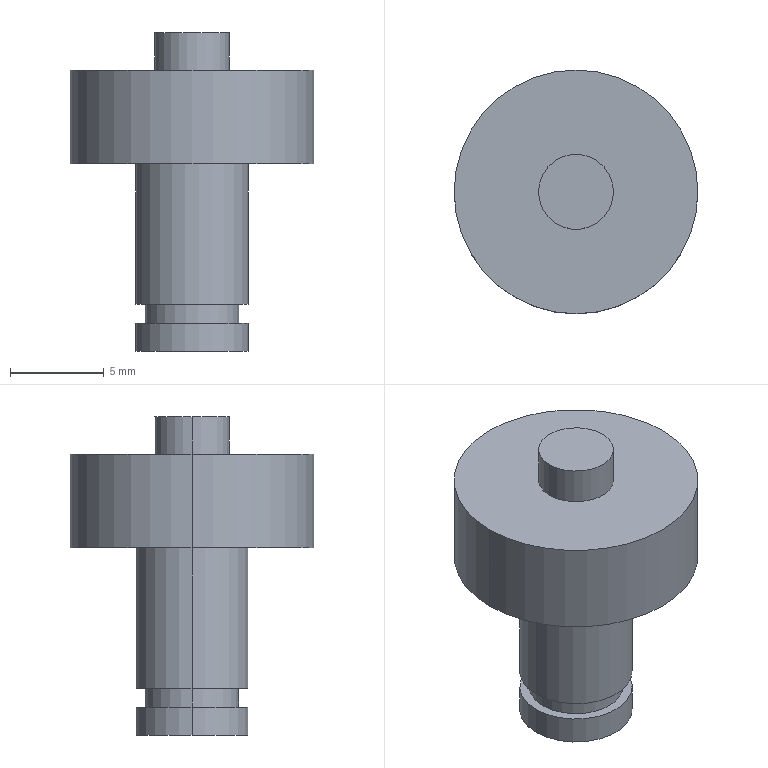Part | SolidWorks | features Boss 4, Extrusion 1 | 1 solid | 16 faces | box 13 x 13 x 17 mm | volume 962.898 mm3 | cylinder 10 | plane 6 | commonest cylinder face diameters 6 x4 4 x2 5 x2 13 x2
STEP:
#1=CARTESIAN_POINT('',(-3.,0.,-10.));
#2=VERTEX_POINT('',#1);
#3=CARTESIAN_POINT('',(3.,0.,-10.));
#4=VERTEX_POINT('',#3);
#5=CARTESIAN_POINT('',(0.,0.,-10.));
#6=DIRECTION('',(0.,0.,-1.));
#7=DIRECTION('',(-1.,0.,0.));
#8=AXIS2_PLACEMENT_3D('',#5,#6,#7);
#9=CIRCLE('',#8,3.);
#10=EDGE_CURVE('',#2,#4,#9,.T.);
#11=ORIENTED_EDGE('',*,*,#10,.F.);
#12=CARTESIAN_POINT('',(-3.,0.,-8.5));
#13=VERTEX_POINT('',#12);
#14=CARTESIAN_POINT('',(-3.,0.,-10.));
#15=DIRECTION('',(0.,0.,1.));
#16=VECTOR('',#15,1000.);
#17=LINE('',#14,#16);
#18=EDGE_CURVE('',#2,#13,#17,.T.);
#19=ORIENTED_EDGE('',*,*,#18,.T.);
#20=CARTESIAN_POINT('',(3.,0.,-8.5));
#21=VERTEX_POINT('',#20);
#22=CARTESIAN_POINT('',(0.,0.,-8.5));
#23=DIRECTION('',(0.,0.,-1.));
#24=DIRECTION('',(-1.,0.,0.));
#25=AXIS2_PLACEMENT_3D('',#22,#23,#24);
#26=CIRCLE('',#25,3.);
#27=EDGE_CURVE('',#13,#21,#26,.T.);
#28=ORIENTED_EDGE('',*,*,#27,.T.);
#29=CARTESIAN_POINT('',(3.,0.,-10.));
#30=DIRECTION('',(0.,0.,1.));
#31=VECTOR('',#30,1000.);
#32=LINE('',#29,#31);
#33=EDGE_CURVE('',#4,#21,#32,.T.);
#34=ORIENTED_EDGE('',*,*,#33,.F.);
#35=EDGE_LOOP('',(#11,#19,#28,#34));
#36=FACE_OUTER_BOUND('',#35,.T.);
#37=CARTESIAN_POINT('',(0.,0.,-10.));
#38=DIRECTION('',(0.,0.,1.));
#39=DIRECTION('',(1.,0.,0.));
#40=AXIS2_PLACEMENT_3D('',#37,#38,#39);
#41=CYLINDRICAL_SURFACE('',#40,3.);
#42=ADVANCED_FACE('',(#36),#41,.T.);
#43=CARTESIAN_POINT('',(-2.5,0.,-8.5));
#44=VERTEX_POINT('',#43);
#45=CARTESIAN_POINT('',(2.5,0.,-8.5));
#46=VERTEX_POINT('',#45);
#47=CARTESIAN_POINT('',(0.,0.,-8.5));
#48=DIRECTION('',(0.,0.,-1.));
#49=DIRECTION('',(-1.,0.,0.));
#50=AXIS2_PLACEMENT_3D('',#47,#48,#49);
#51=CIRCLE('',#50,2.5);
#52=EDGE_CURVE('',#44,#46,#51,.T.);
#53=ORIENTED_EDGE('',*,*,#52,.F.);
#54=CARTESIAN_POINT('',(-2.5,0.,-7.5));
#55=VERTEX_POINT('',#54);
#56=CARTESIAN_POINT('',(-2.5,0.,-8.5));
#57=DIRECTION('',(0.,0.,1.));
#58=VECTOR('',#57,1000.);
#59=LINE('',#56,#58);
#60=EDGE_CURVE('',#44,#55,#59,.T.);
#61=ORIENTED_EDGE('',*,*,#60,.T.);
#62=CARTESIAN_POINT('',(2.5,0.,-7.5));
#63=VERTEX_POINT('',#62);
#64=CARTESIAN_POINT('',(0.,0.,-7.5));
#65=DIRECTION('',(0.,0.,-1.));
#66=DIRECTION('',(-1.,0.,0.));
#67=AXIS2_PLACEMENT_3D('',#64,#65,#66);
#68=CIRCLE('',#67,2.5);
#69=EDGE_CURVE('',#55,#63,#68,.T.);
#70=ORIENTED_EDGE('',*,*,#69,.T.);
#71=CARTESIAN_POINT('',(2.5,0.,-8.5));
#72=DIRECTION('',(0.,0.,1.));
#73=VECTOR('',#72,1000.);
#74=LINE('',#71,#73);
#75=EDGE_CURVE('',#46,#63,#74,.T.);
#76=ORIENTED_EDGE('',*,*,#75,.F.);
#77=EDGE_LOOP('',(#53,#61,#70,#76));
#78=FACE_OUTER_BOUND('',#77,.T.);
#79=CARTESIAN_POINT('',(0.,0.,-8.5));
#80=DIRECTION('',(0.,0.,1.));
#81=DIRECTION('',(1.,0.,0.));
#82=AXIS2_PLACEMENT_3D('',#79,#80,#81);
#83=CYLINDRICAL_SURFACE('',#82,2.5);
#84=ADVANCED_FACE('',(#78),#83,.T.);
#85=CARTESIAN_POINT('',(-3.,0.,-7.5));
#86=VERTEX_POINT('',#85);
#87=CARTESIAN_POINT('',(3.,0.,-7.5));
#88=VERTEX_POINT('',#87);
#89=CARTESIAN_POINT('',(0.,0.,-7.5));
#90=DIRECTION('',(0.,0.,-1.));
#91=DIRECTION('',(-1.,0.,0.));
#92=AXIS2_PLACEMENT_3D('',#89,#90,#91);
#93=CIRCLE('',#92,3.);
#94=EDGE_CURVE('',#86,#88,#93,.T.);
#95=ORIENTED_EDGE('',*,*,#94,.F.);
#96=CARTESIAN_POINT('',(-3.,0.,0.));
#97=VERTEX_POINT('',#96);
#98=CARTESIAN_POINT('',(-3.,0.,-7.5));
#99=DIRECTION('',(0.,0.,1.));
#100=VECTOR('',#99,1000.);
#101=LINE('',#98,#100);
#102=EDGE_CURVE('',#86,#97,#101,.T.);
#103=ORIENTED_EDGE('',*,*,#102,.T.);
#104=CARTESIAN_POINT('',(3.,0.,0.));
#105=VERTEX_POINT('',#104);
#106=CARTESIAN_POINT('',(0.,0.,0.));
#107=DIRECTION('',(0.,0.,-1.));
#108=DIRECTION('',(1.,0.,0.));
#109=AXIS2_PLACEMENT_3D('',#106,#107,#108);
#110=CIRCLE('',#109,3.);
#111=EDGE_CURVE('',#97,#105,#110,.T.);
#112=ORIENTED_EDGE('',*,*,#111,.T.);
#113=CARTESIAN_POINT('',(3.,0.,-7.5));
#114=DIRECTION('',(0.,0.,1.));
#115=VECTOR('',#114,1000.);
#116=LINE('',#113,#115);
#117=EDGE_CURVE('',#88,#105,#116,.T.);
#118=ORIENTED_EDGE('',*,*,#117,.F.);
#119=EDGE_LOOP('',(#95,#103,#112,#118));
#120=FACE_OUTER_BOUND('',#119,.T.);
#121=CARTESIAN_POINT('',(0.,0.,-7.5));
#122=DIRECTION('',(0.,0.,1.));
#123=DIRECTION('',(1.,0.,0.));
#124=AXIS2_PLACEMENT_3D('',#121,#122,#123);
#125=CYLINDRICAL_SURFACE('',#124,3.);
#126=ADVANCED_FACE('',(#120),#125,.T.);
#127=CARTESIAN_POINT('',(2.,0.,7.));
#128=VERTEX_POINT('',#127);
#129=CARTESIAN_POINT('',(-2.,0.,7.));
#130=VERTEX_POINT('',#129);
#131=CARTESIAN_POINT('',(0.,0.,7.));
#132=DIRECTION('',(0.,0.,1.));
#133=DIRECTION('',(1.,0.,0.));
#134=AXIS2_PLACEMENT_3D('',#131,#132,#133);
#135=CIRCLE('',#134,2.);
#136=EDGE_CURVE('',#128,#130,#135,.T.);
#137=ORIENTED_EDGE('',*,*,#136,.F.);
#138=CARTESIAN_POINT('',(2.,0.,5.));
#139=VERTEX_POINT('',#138);
#140=CARTESIAN_POINT('',(2.,0.,7.));
#141=DIRECTION('',(0.,0.,-1.));
#142=VECTOR('',#141,1000.);
#143=LINE('',#140,#142);
#144=EDGE_CURVE('',#128,#139,#143,.T.);
#145=ORIENTED_EDGE('',*,*,#144,.T.);
#146=CARTESIAN_POINT('',(-2.,0.,5.));
#147=VERTEX_POINT('',#146);
#148=CARTESIAN_POINT('',(0.,0.,5.));
#149=DIRECTION('',(0.,0.,1.));
#150=DIRECTION('',(1.,0.,0.));
#151=AXIS2_PLACEMENT_3D('',#148,#149,#150);
#152=CIRCLE('',#151,2.);
#153=EDGE_CURVE('',#139,#147,#152,.T.);
#154=ORIENTED_EDGE('',*,*,#153,.T.);
#155=CARTESIAN_POINT('',(-2.,0.,7.));
#156=DIRECTION('',(0.,0.,-1.));
#157=VECTOR('',#156,1000.);
#158=LINE('',#155,#157);
#159=EDGE_CURVE('',#130,#147,#158,.T.);
#160=ORIENTED_EDGE('',*,*,#159,.F.);
#161=EDGE_LOOP('',(#137,#145,#154,#160));
#162=FACE_OUTER_BOUND('',#161,.T.);
#163=CARTESIAN_POINT('',(0.,0.,7.));
#164=DIRECTION('',(0.,0.,-1.));
#165=DIRECTION('',(-1.,0.,0.));
#166=AXIS2_PLACEMENT_3D('',#163,#164,#165);
#167=CYLINDRICAL_SURFACE('',#166,2.);
#168=ADVANCED_FACE('',(#162),#167,.T.);
#169=CARTESIAN_POINT('',(6.5,0.,5.));
#170=VERTEX_POINT('',#169);
#171=CARTESIAN_POINT('',(-6.5,0.,5.));
#172=VERTEX_POINT('',#171);
#173=CARTESIAN_POINT('',(0.,0.,5.));
#174=DIRECTION('',(0.,0.,1.));
#175=DIRECTION('',(1.,0.,0.));
#176=AXIS2_PLACEMENT_3D('',#173,#174,#175);
#177=CIRCLE('',#176,6.5);
#178=EDGE_CURVE('',#170,#172,#177,.T.);
#179=ORIENTED_EDGE('',*,*,#178,.F.);
#180=CARTESIAN_POINT('',(6.5,0.,0.));
#181=VERTEX_POINT('',#180);
#182=CARTESIAN_POINT('',(6.5,0.,5.));
#183=DIRECTION('',(0.,0.,-1.));
#184=VECTOR('',#183,1000.);
#185=LINE('',#182,#184);
#186=EDGE_CURVE('',#170,#181,#185,.T.);
#187=ORIENTED_EDGE('',*,*,#186,.T.);
#188=CARTESIAN_POINT('',(-6.5,0.,0.));
#189=VERTEX_POINT('',#188);
#190=CARTESIAN_POINT('',(0.,0.,0.));
#191=DIRECTION('',(0.,0.,1.));
#192=DIRECTION('',(1.,0.,0.));
#193=AXIS2_PLACEMENT_3D('',#190,#191,#192);
#194=CIRCLE('',#193,6.5);
#195=EDGE_CURVE('',#181,#189,#194,.T.);
#196=ORIENTED_EDGE('',*,*,#195,.T.);
#197=CARTESIAN_POINT('',(-6.5,0.,5.));
#198=DIRECTION('',(0.,0.,-1.));
#199=VECTOR('',#198,1000.);
#200=LINE('',#197,#199);
#201=EDGE_CURVE('',#172,#189,#200,.T.);
#202=ORIENTED_EDGE('',*,*,#201,.F.);
#203=EDGE_LOOP('',(#179,#187,#196,#202));
#204=FACE_OUTER_BOUND('',#203,.T.);
#205=CARTESIAN_POINT('',(0.,0.,5.));
#206=DIRECTION('',(0.,0.,-1.));
#207=DIRECTION('',(-1.,0.,0.));
#208=AXIS2_PLACEMENT_3D('',#205,#206,#207);
#209=CYLINDRICAL_SURFACE('',#208,6.5);
#210=ADVANCED_FACE('',(#204),#209,.T.);
#211=CARTESIAN_POINT('',(0.,0.,-7.5));
#212=DIRECTION('',(0.,0.,-1.));
#213=DIRECTION('',(-1.,0.,0.));
#214=AXIS2_PLACEMENT_3D('',#211,#212,#213);
#215=CIRCLE('',#214,3.);
#216=EDGE_CURVE('',#88,#86,#215,.T.);
#217=ORIENTED_EDGE('',*,*,#216,.T.);
#218=ORIENTED_EDGE('',*,*,#94,.T.);
#219=EDGE_LOOP('',(#217,#218));
#220=FACE_OUTER_BOUND('',#219,.T.);
#221=CARTESIAN_POINT('',(0.,0.,-7.5));
#222=DIRECTION('',(0.,0.,-1.));
#223=DIRECTION('',(-1.,0.,0.));
#224=AXIS2_PLACEMENT_3D('',#221,#222,#223);
#225=CIRCLE('',#224,2.5);
#226=EDGE_CURVE('',#63,#55,#225,.T.);
#227=ORIENTED_EDGE('',*,*,#226,.F.);
#228=ORIENTED_EDGE('',*,*,#69,.F.);
#229=EDGE_LOOP('',(#227,#228));
#230=FACE_BOUND('',#229,.T.);
#231=CARTESIAN_POINT('',(0.,0.,-7.5));
#232=DIRECTION('',(0.,0.,-1.));
#233=DIRECTION('',(-1.,0.,0.));
#234=AXIS2_PLACEMENT_3D('',#231,#232,#233);
#235=PLANE('',#234);
#236=ADVANCED_FACE('',(#220,#230),#235,.T.);
#237=CARTESIAN_POINT('',(0.,0.,0.));
#238=DIRECTION('',(0.,0.,1.));
#239=DIRECTION('',(1.,0.,0.));
#240=AXIS2_PLACEMENT_3D('',#237,#238,#239);
#241=CIRCLE('',#240,6.5);
#242=EDGE_CURVE('',#189,#181,#241,.T.);
#243=ORIENTED_EDGE('',*,*,#242,.F.);
#244=ORIENTED_EDGE('',*,*,#195,.F.);
#245=EDGE_LOOP('',(#243,#244));
#246=FACE_OUTER_BOUND('',#245,.T.);
#247=CARTESIAN_POINT('',(0.,0.,0.));
#248=DIRECTION('',(0.,0.,-1.));
#249=DIRECTION('',(1.,0.,0.));
#250=AXIS2_PLACEMENT_3D('',#247,#248,#249);
#251=CIRCLE('',#250,3.);
#252=EDGE_CURVE('',#105,#97,#251,.T.);
#253=ORIENTED_EDGE('',*,*,#252,.F.);
#254=ORIENTED_EDGE('',*,*,#111,.F.);
#255=EDGE_LOOP('',(#253,#254));
#256=FACE_BOUND('',#255,.T.);
#257=CARTESIAN_POINT('',(0.,0.,0.));
#258=DIRECTION('',(0.,0.,1.));
#259=DIRECTION('',(1.,0.,0.));
#260=AXIS2_PLACEMENT_3D('',#257,#258,#259);
#261=PLANE('',#260);
#262=ADVANCED_FACE('',(#246,#256),#261,.F.);
#263=CARTESIAN_POINT('',(0.,0.,5.));
#264=DIRECTION('',(0.,0.,1.));
#265=DIRECTION('',(1.,0.,0.));
#266=AXIS2_PLACEMENT_3D('',#263,#264,#265);
#267=CIRCLE('',#266,6.5);
#268=EDGE_CURVE('',#172,#170,#267,.T.);
#269=ORIENTED_EDGE('',*,*,#268,.T.);
#270=ORIENTED_EDGE('',*,*,#178,.T.);
#271=EDGE_LOOP('',(#269,#270));
#272=FACE_OUTER_BOUND('',#271,.T.);
#273=CARTESIAN_POINT('',(0.,0.,5.));
#274=DIRECTION('',(0.,0.,1.));
#275=DIRECTION('',(1.,0.,0.));
#276=AXIS2_PLACEMENT_3D('',#273,#274,#275);
#277=CIRCLE('',#276,2.);
#278=EDGE_CURVE('',#147,#139,#277,.T.);
#279=ORIENTED_EDGE('',*,*,#278,.F.);
#280=ORIENTED_EDGE('',*,*,#153,.F.);
#281=EDGE_LOOP('',(#279,#280));
#282=FACE_BOUND('',#281,.T.);
#283=CARTESIAN_POINT('',(0.,0.,5.));
#284=DIRECTION('',(0.,0.,1.));
#285=DIRECTION('',(1.,0.,0.));
#286=AXIS2_PLACEMENT_3D('',#283,#284,#285);
#287=PLANE('',#286);
#288=ADVANCED_FACE('',(#272,#282),#287,.T.);
#289=ORIENTED_EDGE('',*,*,#186,.F.);
#290=ORIENTED_EDGE('',*,*,#268,.F.);
#291=ORIENTED_EDGE('',*,*,#201,.T.);
#292=ORIENTED_EDGE('',*,*,#242,.T.);
#293=EDGE_LOOP('',(#289,#290,#291,#292));
#294=FACE_OUTER_BOUND('',#293,.T.);
#295=CARTESIAN_POINT('',(0.,0.,5.));
#296=DIRECTION('',(0.,0.,-1.));
#297=DIRECTION('',(-1.,0.,0.));
#298=AXIS2_PLACEMENT_3D('',#295,#296,#297);
#299=CYLINDRICAL_SURFACE('',#298,6.5);
#300=ADVANCED_FACE('',(#294),#299,.T.);
#301=ORIENTED_EDGE('',*,*,#144,.F.);
#302=CARTESIAN_POINT('',(0.,0.,7.));
#303=DIRECTION('',(0.,0.,1.));
#304=DIRECTION('',(1.,0.,0.));
#305=AXIS2_PLACEMENT_3D('',#302,#303,#304);
#306=CIRCLE('',#305,2.);
#307=EDGE_CURVE('',#130,#128,#306,.T.);
#308=ORIENTED_EDGE('',*,*,#307,.F.);
#309=ORIENTED_EDGE('',*,*,#159,.T.);
#310=ORIENTED_EDGE('',*,*,#278,.T.);
#311=EDGE_LOOP('',(#301,#308,#309,#310));
#312=FACE_OUTER_BOUND('',#311,.T.);
#313=CARTESIAN_POINT('',(0.,0.,7.));
#314=DIRECTION('',(0.,0.,-1.));
#315=DIRECTION('',(-1.,0.,0.));
#316=AXIS2_PLACEMENT_3D('',#313,#314,#315);
#317=CYLINDRICAL_SURFACE('',#316,2.);
#318=ADVANCED_FACE('',(#312),#317,.T.);
#319=ORIENTED_EDGE('',*,*,#307,.T.);
#320=ORIENTED_EDGE('',*,*,#136,.T.);
#321=EDGE_LOOP('',(#319,#320));
#322=FACE_OUTER_BOUND('',#321,.T.);
#323=CARTESIAN_POINT('',(0.,0.,7.));
#324=DIRECTION('',(0.,0.,1.));
#325=DIRECTION('',(1.,0.,0.));
#326=AXIS2_PLACEMENT_3D('',#323,#324,#325);
#327=PLANE('',#326);
#328=ADVANCED_FACE('',(#322),#327,.T.);
#329=ORIENTED_EDGE('',*,*,#102,.F.);
#330=ORIENTED_EDGE('',*,*,#216,.F.);
#331=ORIENTED_EDGE('',*,*,#117,.T.);
#332=ORIENTED_EDGE('',*,*,#252,.T.);
#333=EDGE_LOOP('',(#329,#330,#331,#332));
#334=FACE_OUTER_BOUND('',#333,.T.);
#335=CARTESIAN_POINT('',(0.,0.,-7.5));
#336=DIRECTION('',(0.,0.,1.));
#337=DIRECTION('',(1.,0.,0.));
#338=AXIS2_PLACEMENT_3D('',#335,#336,#337);
#339=CYLINDRICAL_SURFACE('',#338,3.);
#340=ADVANCED_FACE('',(#334),#339,.T.);
#341=ORIENTED_EDGE('',*,*,#60,.F.);
#342=CARTESIAN_POINT('',(0.,0.,-8.5));
#343=DIRECTION('',(0.,0.,-1.));
#344=DIRECTION('',(-1.,0.,0.));
#345=AXIS2_PLACEMENT_3D('',#342,#343,#344);
#346=CIRCLE('',#345,2.5);
#347=EDGE_CURVE('',#46,#44,#346,.T.);
#348=ORIENTED_EDGE('',*,*,#347,.F.);
#349=ORIENTED_EDGE('',*,*,#75,.T.);
#350=ORIENTED_EDGE('',*,*,#226,.T.);
#351=EDGE_LOOP('',(#341,#348,#349,#350));
#352=FACE_OUTER_BOUND('',#351,.T.);
#353=CARTESIAN_POINT('',(0.,0.,-8.5));
#354=DIRECTION('',(0.,0.,1.));
#355=DIRECTION('',(1.,0.,0.));
#356=AXIS2_PLACEMENT_3D('',#353,#354,#355);
#357=CYLINDRICAL_SURFACE('',#356,2.5);
#358=ADVANCED_FACE('',(#352),#357,.T.);
#359=CARTESIAN_POINT('',(0.,0.,-8.5));
#360=DIRECTION('',(0.,0.,-1.));
#361=DIRECTION('',(-1.,0.,0.));
#362=AXIS2_PLACEMENT_3D('',#359,#360,#361);
#363=CIRCLE('',#362,3.);
#364=EDGE_CURVE('',#21,#13,#363,.T.);
#365=ORIENTED_EDGE('',*,*,#364,.F.);
#366=ORIENTED_EDGE('',*,*,#27,.F.);
#367=EDGE_LOOP('',(#365,#366));
#368=FACE_OUTER_BOUND('',#367,.T.);
#369=ORIENTED_EDGE('',*,*,#347,.T.);
#370=ORIENTED_EDGE('',*,*,#52,.T.);
#371=EDGE_LOOP('',(#369,#370));
#372=FACE_BOUND('',#371,.T.);
#373=CARTESIAN_POINT('',(0.,0.,-8.5));
#374=DIRECTION('',(0.,0.,-1.));
#375=DIRECTION('',(-1.,0.,0.));
#376=AXIS2_PLACEMENT_3D('',#373,#374,#375);
#377=PLANE('',#376);
#378=ADVANCED_FACE('',(#368,#372),#377,.F.);
#379=ORIENTED_EDGE('',*,*,#18,.F.);
#380=CARTESIAN_POINT('',(0.,0.,-10.));
#381=DIRECTION('',(0.,0.,-1.));
#382=DIRECTION('',(-1.,0.,0.));
#383=AXIS2_PLACEMENT_3D('',#380,#381,#382);
#384=CIRCLE('',#383,3.);
#385=EDGE_CURVE('',#4,#2,#384,.T.);
#386=ORIENTED_EDGE('',*,*,#385,.F.);
#387=ORIENTED_EDGE('',*,*,#33,.T.);
#388=ORIENTED_EDGE('',*,*,#364,.T.);
#389=EDGE_LOOP('',(#379,#386,#387,#388));
#390=FACE_OUTER_BOUND('',#389,.T.);
#391=CARTESIAN_POINT('',(0.,0.,-10.));
#392=DIRECTION('',(0.,0.,1.));
#393=DIRECTION('',(1.,0.,0.));
#394=AXIS2_PLACEMENT_3D('',#391,#392,#393);
#395=CYLINDRICAL_SURFACE('',#394,3.);
#396=ADVANCED_FACE('',(#390),#395,.T.);
#397=ORIENTED_EDGE('',*,*,#385,.T.);
#398=ORIENTED_EDGE('',*,*,#10,.T.);
#399=EDGE_LOOP('',(#397,#398));
#400=FACE_OUTER_BOUND('',#399,.T.);
#401=CARTESIAN_POINT('',(0.,0.,-10.));
#402=DIRECTION('',(0.,0.,-1.));
#403=DIRECTION('',(-1.,0.,0.));
#404=AXIS2_PLACEMENT_3D('',#401,#402,#403);
#405=PLANE('',#404);
#406=ADVANCED_FACE('',(#400),#405,.T.);
#407=CLOSED_SHELL('',(#42,#84,#126,#168,#210,#236,#262,#288,#300,#318,#328,#340,#358,#378,#396,#406));
#408=MANIFOLD_SOLID_BREP('',#407);
#409=CARTESIAN_POINT('',(0.,0.,0.));
#410=DIRECTION('',(0.,0.,1.));
#411=DIRECTION('',(1.,0.,0.));
#412=AXIS2_PLACEMENT_3D('',#409,#410,#411);
#413=(LENGTH_UNIT()NAMED_UNIT(*)SI_UNIT(.MILLI.,.METRE.));
#414=UNCERTAINTY_MEASURE_WITH_UNIT(LENGTH_MEASURE(0.00001),#413,'','');
#415=(NAMED_UNIT(*)PLANE_ANGLE_UNIT()SI_UNIT($,.RADIAN.));
#416=(NAMED_UNIT(*)SI_UNIT($,.STERADIAN.)SOLID_ANGLE_UNIT());
#417=(GEOMETRIC_REPRESENTATION_CONTEXT(3)GLOBAL_UNCERTAINTY_ASSIGNED_CONTEXT((#414))GLOBAL_UNIT_ASSIGNED_CONTEXT((#413,#415,#416))REPRESENTATION_CONTEXT('',''));
#418=ADVANCED_BREP_SHAPE_REPRESENTATION('',(#408,#412),#417);